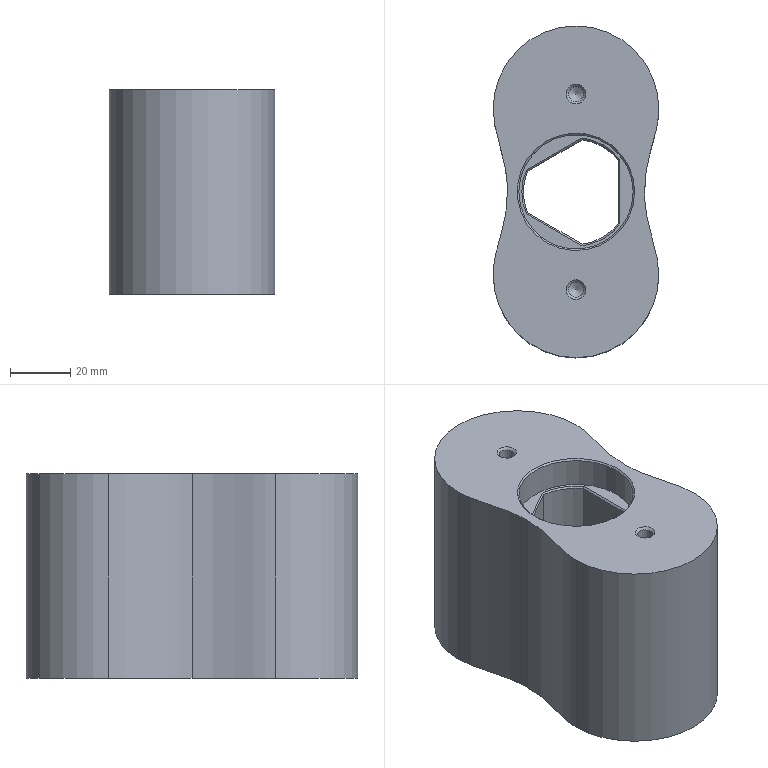NC program | NX | posted with a generic post | part box 55.004 x 110.159 x 68 mm
Lines 17733 to 17802 of 17802:
(PLANAR_MILL_COPY_COPY_COPY , TOOL : D6A45)
N35452 T07 M6
N35454 G54
N35456 G17 G0 G90 X-20.492 Y-0.096 S7500 M3
N35458 G43 Z30. H7
N35460 Z1.5
N35462 G94 G1 Z-1.5 F1250.
N35464 G3 X-20.25 Y0.25 R0.5
N35466 X-20.5 Y0. R0.25
N35468 X-20.25 Y0.25 R-0.25
N35470 X-20.008 Y-0.096 R0.5
N35472 G1 Z1.5
N35474 G0 Z30.
N35476 X0.766 Y16.943
N35478 Z1.5
N35480 G1 Z-1.5
N35482 G3 X0. Y17.3 R1.
N35484 X-17.3 Y0. R17.3
N35486 X0. Y17.3 R-17.3
N35488 X-0.766 Y16.943 R1.
N35490 G1 Z1.5
N35492 G0 Z30.
N35494 X-0.767 Y24.127
N35496 Z1.5
N35498 G1 Z-1.5
N35500 G3 X0. Y23.771 R1.
N35502 X5.127 Y24.082 R43.463
N35504 X10.212 Y24.953 R51.868
N35506 X14.567 Y26.072 R69.703
N35508 G2 X18.998 Y27.289 R145.723
N35510 X23.225 Y28.162 R44.344
N35512 X27.577 Y28.502 R28.394
N35514 X56.079 Y0. R28.502
N35516 X27.576 Y-28.502 R28.502
N35518 X23.144 Y-28.149 R28.378
N35520 X18.843 Y-27.249 R45.449
N35522 X14.497 Y-26.052 R159.504
N35524 G3 X10.222 Y-24.955 R69.611
N35526 X5.132 Y-24.083 R51.893
N35528 X0. Y-23.771 R43.462
N35530 X-5.127 Y-24.082 R43.463
N35532 X-10.212 Y-24.953 R51.868
N35534 X-14.567 Y-26.072 R69.703
N35536 G2 X-18.998 Y-27.289 R145.723
N35538 X-23.225 Y-28.162 R44.344
N35540 X-27.577 Y-28.502 R28.394
N35542 X-56.079 Y0. R28.502
N35544 X-27.576 Y28.502 R28.502
N35546 X-23.144 Y28.149 R28.378
N35548 X-18.843 Y27.249 R45.449
N35550 X-14.497 Y26.052 R159.504
N35552 G3 X-10.222 Y24.955 R69.611
N35554 X-5.132 Y24.083 R51.893
N35556 X0. Y23.771 R43.462
N35558 X0.766 Y24.129 R1.
N35560 G1 Z1.5
N35562 G0 Z30.
N35564 X20.008 Y-0.096
N35566 Z1.5
N35568 G1 Z-1.5
N35570 G3 X20.25 Y0.25 R0.5
N35572 X20. Y0. R0.25
N35574 X20.25 Y0.25 R-0.25
N35576 X20.492 Y-0.096 R0.5
N35578 G1 Z1.5
N35580 G0 Z30.
N35582 M5
N35584 M2